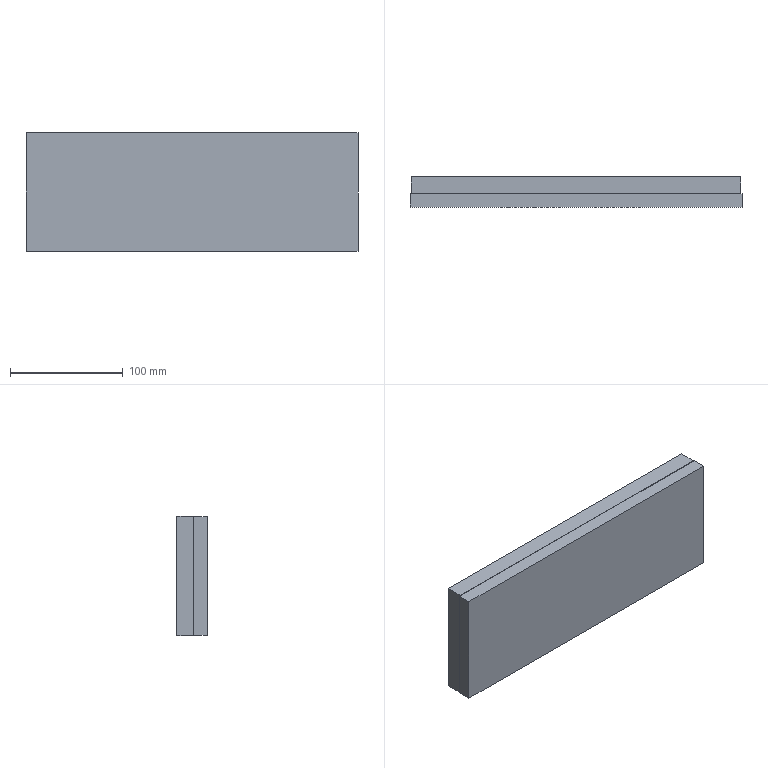Part | 5 solids | 145 faces | box 295 x 27 x 106 mm | volume 1564889 mm3 | plane 77 | cylinder 56 | cone 12 | commonest cylinder face diameters 6.6 x12 10 x12 20 x12 5 x6 6 x6 4 x2